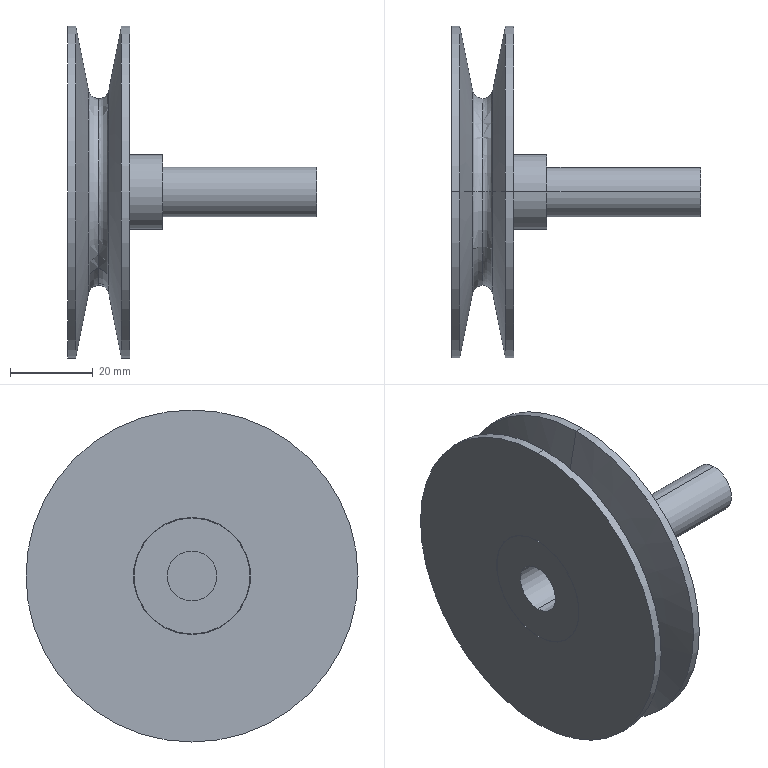Part | SolidWorks | features ICE 5, Revolution 1 | 1 solid | 35 faces | box 60 x 80 x 80 mm | volume 53043 mm3 | cylinder 18 | plane 9 | torus 4 | cone 4 | commonest cylinder face diameters 12 x4 28 x4 28.2 x4 80 x4 18 x2
STEP:
#1=CARTESIAN_POINT('',(5.047,0.,24.517));
#2=VERTEX_POINT('',#1);
#3=CARTESIAN_POINT('',(7.5,0.,22.5));
#4=VERTEX_POINT('',#3);
#5=CARTESIAN_POINT('',(7.5,0.,25.));
#6=DIRECTION('',(0.,-1.,0.));
#7=DIRECTION('',(0.,0.,-1.));
#8=AXIS2_PLACEMENT_3D('',#5,#6,#7);
#9=CIRCLE('',#8,2.5);
#10=EDGE_CURVE('',#2,#4,#9,.T.);
#11=ORIENTED_EDGE('',*,*,#10,.T.);
#12=CARTESIAN_POINT('',(7.5,0.,-22.5));
#13=VERTEX_POINT('',#12);
#14=CARTESIAN_POINT('',(7.5,0.,0.));
#15=DIRECTION('',(-1.,0.,0.));
#16=DIRECTION('',(0.,0.,1.));
#17=AXIS2_PLACEMENT_3D('',#14,#15,#16);
#18=CIRCLE('',#17,22.5);
#19=EDGE_CURVE('',#4,#13,#18,.T.);
#20=ORIENTED_EDGE('',*,*,#19,.T.);
#21=CARTESIAN_POINT('',(5.047,0.,-24.517));
#22=VERTEX_POINT('',#21);
#23=CARTESIAN_POINT('',(7.5,0.,-25.));
#24=DIRECTION('',(0.,1.,0.));
#25=DIRECTION('',(0.,0.,1.));
#26=AXIS2_PLACEMENT_3D('',#23,#24,#25);
#27=CIRCLE('',#26,2.5);
#28=EDGE_CURVE('',#22,#13,#27,.T.);
#29=ORIENTED_EDGE('',*,*,#28,.F.);
#30=CARTESIAN_POINT('',(5.047,0.,0.));
#31=DIRECTION('',(-1.,0.,0.));
#32=DIRECTION('',(0.,0.,1.));
#33=AXIS2_PLACEMENT_3D('',#30,#31,#32);
#34=CIRCLE('',#33,24.517);
#35=EDGE_CURVE('',#2,#22,#34,.T.);
#36=ORIENTED_EDGE('',*,*,#35,.F.);
#37=EDGE_LOOP('',(#11,#20,#29,#36));
#38=FACE_OUTER_BOUND('',#37,.T.);
#39=CARTESIAN_POINT('',(7.5,0.,0.));
#40=DIRECTION('',(-1.,0.,0.));
#41=DIRECTION('',(0.,0.,1.));
#42=AXIS2_PLACEMENT_3D('',#39,#40,#41);
#43=TOROIDAL_SURFACE('',#42,25.,2.5);
#44=ADVANCED_FACE('',(#38),#43,.F.);
#45=ORIENTED_EDGE('',*,*,#28,.T.);
#46=CARTESIAN_POINT('',(7.5,0.,0.));
#47=DIRECTION('',(-1.,0.,0.));
#48=DIRECTION('',(0.,0.,1.));
#49=AXIS2_PLACEMENT_3D('',#46,#47,#48);
#50=CIRCLE('',#49,22.5);
#51=EDGE_CURVE('',#13,#4,#50,.T.);
#52=ORIENTED_EDGE('',*,*,#51,.T.);
#53=ORIENTED_EDGE('',*,*,#10,.F.);
#54=CARTESIAN_POINT('',(5.047,0.,0.));
#55=DIRECTION('',(-1.,0.,0.));
#56=DIRECTION('',(0.,0.,1.));
#57=AXIS2_PLACEMENT_3D('',#54,#55,#56);
#58=CIRCLE('',#57,24.517);
#59=EDGE_CURVE('',#22,#2,#58,.T.);
#60=ORIENTED_EDGE('',*,*,#59,.F.);
#61=EDGE_LOOP('',(#45,#52,#53,#60));
#62=FACE_OUTER_BOUND('',#61,.T.);
#63=CARTESIAN_POINT('',(7.5,0.,0.));
#64=DIRECTION('',(-1.,0.,0.));
#65=DIRECTION('',(0.,0.,1.));
#66=AXIS2_PLACEMENT_3D('',#63,#64,#65);
#67=TOROIDAL_SURFACE('',#66,25.,2.5);
#68=ADVANCED_FACE('',(#62),#67,.F.);
#69=CARTESIAN_POINT('',(60.,0.,-6.));
#70=VERTEX_POINT('',#69);
#71=CARTESIAN_POINT('',(60.,0.,6.));
#72=VERTEX_POINT('',#71);
#73=CARTESIAN_POINT('',(60.,0.,0.));
#74=DIRECTION('',(1.,0.,0.));
#75=DIRECTION('',(0.,0.,-1.));
#76=AXIS2_PLACEMENT_3D('',#73,#74,#75);
#77=CIRCLE('',#76,6.);
#78=EDGE_CURVE('',#70,#72,#77,.T.);
#79=ORIENTED_EDGE('',*,*,#78,.F.);
#80=CARTESIAN_POINT('',(23.,0.,-6.));
#81=VERTEX_POINT('',#80);
#82=CARTESIAN_POINT('',(60.,0.,-6.));
#83=DIRECTION('',(-1.,0.,0.));
#84=VECTOR('',#83,1000.);
#85=LINE('',#82,#84);
#86=EDGE_CURVE('',#70,#81,#85,.T.);
#87=ORIENTED_EDGE('',*,*,#86,.T.);
#88=CARTESIAN_POINT('',(23.,0.,6.));
#89=VERTEX_POINT('',#88);
#90=CARTESIAN_POINT('',(23.,0.,0.));
#91=DIRECTION('',(-1.,0.,0.));
#92=DIRECTION('',(0.,0.,-1.));
#93=AXIS2_PLACEMENT_3D('',#90,#91,#92);
#94=CIRCLE('',#93,6.);
#95=EDGE_CURVE('',#89,#81,#94,.T.);
#96=ORIENTED_EDGE('',*,*,#95,.F.);
#97=CARTESIAN_POINT('',(60.,0.,6.));
#98=DIRECTION('',(-1.,0.,0.));
#99=VECTOR('',#98,1000.);
#100=LINE('',#97,#99);
#101=EDGE_CURVE('',#72,#89,#100,.T.);
#102=ORIENTED_EDGE('',*,*,#101,.F.);
#103=EDGE_LOOP('',(#79,#87,#96,#102));
#104=FACE_OUTER_BOUND('',#103,.T.);
#105=CARTESIAN_POINT('',(60.,0.,0.));
#106=DIRECTION('',(-1.,0.,0.));
#107=DIRECTION('',(0.,0.,1.));
#108=AXIS2_PLACEMENT_3D('',#105,#106,#107);
#109=CYLINDRICAL_SURFACE('',#108,6.);
#110=ADVANCED_FACE('',(#104),#109,.T.);
#111=CARTESIAN_POINT('',(23.,0.,-9.));
#112=VERTEX_POINT('',#111);
#113=CARTESIAN_POINT('',(23.,0.,9.));
#114=VERTEX_POINT('',#113);
#115=CARTESIAN_POINT('',(23.,0.,0.));
#116=DIRECTION('',(1.,0.,0.));
#117=DIRECTION('',(0.,0.,-1.));
#118=AXIS2_PLACEMENT_3D('',#115,#116,#117);
#119=CIRCLE('',#118,9.);
#120=EDGE_CURVE('',#112,#114,#119,.T.);
#121=ORIENTED_EDGE('',*,*,#120,.F.);
#122=CARTESIAN_POINT('',(15.,0.,-9.));
#123=VERTEX_POINT('',#122);
#124=CARTESIAN_POINT('',(23.,0.,-9.));
#125=DIRECTION('',(-1.,0.,0.));
#126=VECTOR('',#125,1000.);
#127=LINE('',#124,#126);
#128=EDGE_CURVE('',#112,#123,#127,.T.);
#129=ORIENTED_EDGE('',*,*,#128,.T.);
#130=CARTESIAN_POINT('',(15.,0.,9.));
#131=VERTEX_POINT('',#130);
#132=CARTESIAN_POINT('',(15.,0.,0.));
#133=DIRECTION('',(1.,0.,0.));
#134=DIRECTION('',(0.,0.,1.));
#135=AXIS2_PLACEMENT_3D('',#132,#133,#134);
#136=CIRCLE('',#135,9.);
#137=EDGE_CURVE('',#123,#131,#136,.T.);
#138=ORIENTED_EDGE('',*,*,#137,.T.);
#139=CARTESIAN_POINT('',(23.,0.,9.));
#140=DIRECTION('',(-1.,0.,0.));
#141=VECTOR('',#140,1000.);
#142=LINE('',#139,#141);
#143=EDGE_CURVE('',#114,#131,#142,.T.);
#144=ORIENTED_EDGE('',*,*,#143,.F.);
#145=EDGE_LOOP('',(#121,#129,#138,#144));
#146=FACE_OUTER_BOUND('',#145,.T.);
#147=CARTESIAN_POINT('',(23.,0.,0.));
#148=DIRECTION('',(-1.,0.,0.));
#149=DIRECTION('',(0.,0.,1.));
#150=AXIS2_PLACEMENT_3D('',#147,#148,#149);
#151=CYLINDRICAL_SURFACE('',#150,9.);
#152=ADVANCED_FACE('',(#146),#151,.T.);
#153=CARTESIAN_POINT('',(12.,0.,-14.));
#154=VERTEX_POINT('',#153);
#155=CARTESIAN_POINT('',(12.,0.,14.));
#156=VERTEX_POINT('',#155);
#157=CARTESIAN_POINT('',(12.,0.,0.));
#158=DIRECTION('',(1.,0.,0.));
#159=DIRECTION('',(0.,0.,-1.));
#160=AXIS2_PLACEMENT_3D('',#157,#158,#159);
#161=CIRCLE('',#160,14.);
#162=EDGE_CURVE('',#154,#156,#161,.T.);
#163=ORIENTED_EDGE('',*,*,#162,.T.);
#164=CARTESIAN_POINT('',(15.,0.,14.));
#165=VERTEX_POINT('',#164);
#166=CARTESIAN_POINT('',(12.,0.,14.));
#167=DIRECTION('',(1.,0.,0.));
#168=VECTOR('',#167,1000.);
#169=LINE('',#166,#168);
#170=EDGE_CURVE('',#156,#165,#169,.T.);
#171=ORIENTED_EDGE('',*,*,#170,.T.);
#172=CARTESIAN_POINT('',(15.,0.,-14.));
#173=VERTEX_POINT('',#172);
#174=CARTESIAN_POINT('',(15.,0.,0.));
#175=DIRECTION('',(1.,0.,0.));
#176=DIRECTION('',(0.,0.,-1.));
#177=AXIS2_PLACEMENT_3D('',#174,#175,#176);
#178=CIRCLE('',#177,14.);
#179=EDGE_CURVE('',#173,#165,#178,.T.);
#180=ORIENTED_EDGE('',*,*,#179,.F.);
#181=CARTESIAN_POINT('',(12.,0.,-14.));
#182=DIRECTION('',(1.,0.,0.));
#183=VECTOR('',#182,1000.);
#184=LINE('',#181,#183);
#185=EDGE_CURVE('',#154,#173,#184,.T.);
#186=ORIENTED_EDGE('',*,*,#185,.F.);
#187=EDGE_LOOP('',(#163,#171,#180,#186));
#188=FACE_OUTER_BOUND('',#187,.T.);
#189=CARTESIAN_POINT('',(12.,0.,0.));
#190=DIRECTION('',(1.,0.,0.));
#191=DIRECTION('',(0.,0.,-1.));
#192=AXIS2_PLACEMENT_3D('',#189,#190,#191);
#193=CYLINDRICAL_SURFACE('',#192,14.);
#194=ADVANCED_FACE('',(#188),#193,.T.);
#195=CARTESIAN_POINT('',(12.,0.,14.1));
#196=VERTEX_POINT('',#195);
#197=CARTESIAN_POINT('',(12.,0.,-14.1));
#198=VERTEX_POINT('',#197);
#199=CARTESIAN_POINT('',(12.,0.,0.));
#200=DIRECTION('',(1.,0.,0.));
#201=DIRECTION('',(0.,0.,-1.));
#202=AXIS2_PLACEMENT_3D('',#199,#200,#201);
#203=CIRCLE('',#202,14.1);
#204=EDGE_CURVE('',#196,#198,#203,.T.);
#205=ORIENTED_EDGE('',*,*,#204,.F.);
#206=CARTESIAN_POINT('',(15.,0.,14.1));
#207=VERTEX_POINT('',#206);
#208=CARTESIAN_POINT('',(12.,0.,14.1));
#209=DIRECTION('',(1.,0.,0.));
#210=VECTOR('',#209,1000.);
#211=LINE('',#208,#210);
#212=EDGE_CURVE('',#196,#207,#211,.T.);
#213=ORIENTED_EDGE('',*,*,#212,.T.);
#214=CARTESIAN_POINT('',(15.,0.,-14.1));
#215=VERTEX_POINT('',#214);
#216=CARTESIAN_POINT('',(15.,0.,0.));
#217=DIRECTION('',(1.,0.,0.));
#218=DIRECTION('',(0.,0.,-1.));
#219=AXIS2_PLACEMENT_3D('',#216,#217,#218);
#220=CIRCLE('',#219,14.1);
#221=EDGE_CURVE('',#207,#215,#220,.T.);
#222=ORIENTED_EDGE('',*,*,#221,.T.);
#223=CARTESIAN_POINT('',(12.,0.,-14.1));
#224=DIRECTION('',(1.,0.,0.));
#225=VECTOR('',#224,1000.);
#226=LINE('',#223,#225);
#227=EDGE_CURVE('',#198,#215,#226,.T.);
#228=ORIENTED_EDGE('',*,*,#227,.F.);
#229=EDGE_LOOP('',(#205,#213,#222,#228));
#230=FACE_OUTER_BOUND('',#229,.T.);
#231=CARTESIAN_POINT('',(12.,0.,0.));
#232=DIRECTION('',(1.,0.,0.));
#233=DIRECTION('',(0.,0.,-1.));
#234=AXIS2_PLACEMENT_3D('',#231,#232,#233);
#235=CYLINDRICAL_SURFACE('',#234,14.1);
#236=ADVANCED_FACE('',(#230),#235,.F.);
#237=CARTESIAN_POINT('',(3.,0.,14.));
#238=VERTEX_POINT('',#237);
#239=CARTESIAN_POINT('',(3.,0.,-14.));
#240=VERTEX_POINT('',#239);
#241=CARTESIAN_POINT('',(3.,0.,0.));
#242=DIRECTION('',(-1.,0.,0.));
#243=DIRECTION('',(0.,0.,1.));
#244=AXIS2_PLACEMENT_3D('',#241,#242,#243);
#245=CIRCLE('',#244,14.);
#246=EDGE_CURVE('',#238,#240,#245,.T.);
#247=ORIENTED_EDGE('',*,*,#246,.T.);
#248=CARTESIAN_POINT('',(0.,0.,-14.));
#249=VERTEX_POINT('',#248);
#250=CARTESIAN_POINT('',(3.,0.,-14.));
#251=DIRECTION('',(-1.,0.,0.));
#252=VECTOR('',#251,1000.);
#253=LINE('',#250,#252);
#254=EDGE_CURVE('',#240,#249,#253,.T.);
#255=ORIENTED_EDGE('',*,*,#254,.T.);
#256=CARTESIAN_POINT('',(0.,0.,14.));
#257=VERTEX_POINT('',#256);
#258=CARTESIAN_POINT('',(0.,0.,0.));
#259=DIRECTION('',(-1.,0.,0.));
#260=DIRECTION('',(0.,0.,1.));
#261=AXIS2_PLACEMENT_3D('',#258,#259,#260);
#262=CIRCLE('',#261,14.);
#263=EDGE_CURVE('',#257,#249,#262,.T.);
#264=ORIENTED_EDGE('',*,*,#263,.F.);
#265=CARTESIAN_POINT('',(3.,0.,14.));
#266=DIRECTION('',(-1.,0.,0.));
#267=VECTOR('',#266,1000.);
#268=LINE('',#265,#267);
#269=EDGE_CURVE('',#238,#257,#268,.T.);
#270=ORIENTED_EDGE('',*,*,#269,.F.);
#271=EDGE_LOOP('',(#247,#255,#264,#270));
#272=FACE_OUTER_BOUND('',#271,.T.);
#273=CARTESIAN_POINT('',(3.,0.,0.));
#274=DIRECTION('',(-1.,0.,0.));
#275=DIRECTION('',(0.,0.,1.));
#276=AXIS2_PLACEMENT_3D('',#273,#274,#275);
#277=CYLINDRICAL_SURFACE('',#276,14.);
#278=ADVANCED_FACE('',(#272),#277,.T.);
#279=CARTESIAN_POINT('',(3.,0.,-14.1));
#280=VERTEX_POINT('',#279);
#281=CARTESIAN_POINT('',(3.,0.,14.1));
#282=VERTEX_POINT('',#281);
#283=CARTESIAN_POINT('',(3.,0.,0.));
#284=DIRECTION('',(-1.,0.,0.));
#285=DIRECTION('',(0.,0.,1.));
#286=AXIS2_PLACEMENT_3D('',#283,#284,#285);
#287=CIRCLE('',#286,14.1);
#288=EDGE_CURVE('',#280,#282,#287,.T.);
#289=ORIENTED_EDGE('',*,*,#288,.F.);
#290=CARTESIAN_POINT('',(0.,0.,-14.1));
#291=VERTEX_POINT('',#290);
#292=CARTESIAN_POINT('',(3.,0.,-14.1));
#293=DIRECTION('',(-1.,0.,0.));
#294=VECTOR('',#293,1000.);
#295=LINE('',#292,#294);
#296=EDGE_CURVE('',#280,#291,#295,.T.);
#297=ORIENTED_EDGE('',*,*,#296,.T.);
#298=CARTESIAN_POINT('',(0.,0.,14.1));
#299=VERTEX_POINT('',#298);
#300=CARTESIAN_POINT('',(0.,0.,0.));
#301=DIRECTION('',(-1.,0.,0.));
#302=DIRECTION('',(0.,0.,1.));
#303=AXIS2_PLACEMENT_3D('',#300,#301,#302);
#304=CIRCLE('',#303,14.1);
#305=EDGE_CURVE('',#291,#299,#304,.T.);
#306=ORIENTED_EDGE('',*,*,#305,.T.);
#307=CARTESIAN_POINT('',(3.,0.,14.1));
#308=DIRECTION('',(-1.,0.,0.));
#309=VECTOR('',#308,1000.);
#310=LINE('',#307,#309);
#311=EDGE_CURVE('',#282,#299,#310,.T.);
#312=ORIENTED_EDGE('',*,*,#311,.F.);
#313=EDGE_LOOP('',(#289,#297,#306,#312));
#314=FACE_OUTER_BOUND('',#313,.T.);
#315=CARTESIAN_POINT('',(3.,0.,0.));
#316=DIRECTION('',(-1.,0.,0.));
#317=DIRECTION('',(0.,0.,1.));
#318=AXIS2_PLACEMENT_3D('',#315,#316,#317);
#319=CYLINDRICAL_SURFACE('',#318,14.1);
#320=ADVANCED_FACE('',(#314),#319,.F.);
#321=CARTESIAN_POINT('',(15.,0.,-6.));
#322=VERTEX_POINT('',#321);
#323=CARTESIAN_POINT('',(15.,0.,6.));
#324=VERTEX_POINT('',#323);
#325=CARTESIAN_POINT('',(15.,0.,0.));
#326=DIRECTION('',(-1.,0.,0.));
#327=DIRECTION('',(0.,0.,1.));
#328=AXIS2_PLACEMENT_3D('',#325,#326,#327);
#329=CIRCLE('',#328,6.);
#330=EDGE_CURVE('',#322,#324,#329,.T.);
#331=ORIENTED_EDGE('',*,*,#330,.F.);
#332=CARTESIAN_POINT('',(0.,0.,-6.));
#333=VERTEX_POINT('',#332);
#334=CARTESIAN_POINT('',(15.,0.,-6.));
#335=DIRECTION('',(-1.,0.,0.));
#336=VECTOR('',#335,1000.);
#337=LINE('',#334,#336);
#338=EDGE_CURVE('',#322,#333,#337,.T.);
#339=ORIENTED_EDGE('',*,*,#338,.T.);
#340=CARTESIAN_POINT('',(0.,0.,6.));
#341=VERTEX_POINT('',#340);
#342=CARTESIAN_POINT('',(0.,0.,0.));
#343=DIRECTION('',(-1.,0.,0.));
#344=DIRECTION('',(0.,0.,1.));
#345=AXIS2_PLACEMENT_3D('',#342,#343,#344);
#346=CIRCLE('',#345,6.);
#347=EDGE_CURVE('',#333,#341,#346,.T.);
#348=ORIENTED_EDGE('',*,*,#347,.T.);
#349=CARTESIAN_POINT('',(15.,0.,6.));
#350=DIRECTION('',(-1.,0.,0.));
#351=VECTOR('',#350,1000.);
#352=LINE('',#349,#351);
#353=EDGE_CURVE('',#324,#341,#352,.T.);
#354=ORIENTED_EDGE('',*,*,#353,.F.);
#355=EDGE_LOOP('',(#331,#339,#348,#354));
#356=FACE_OUTER_BOUND('',#355,.T.);
#357=CARTESIAN_POINT('',(15.,0.,0.));
#358=DIRECTION('',(-1.,0.,0.));
#359=DIRECTION('',(0.,0.,1.));
#360=AXIS2_PLACEMENT_3D('',#357,#358,#359);
#361=CYLINDRICAL_SURFACE('',#360,6.);
#362=ADVANCED_FACE('',(#356),#361,.F.);
#363=CARTESIAN_POINT('',(2.,0.,40.));
#364=VERTEX_POINT('',#363);
#365=CARTESIAN_POINT('',(2.,0.,-40.));
#366=VERTEX_POINT('',#365);
#367=CARTESIAN_POINT('',(2.,0.,0.));
#368=DIRECTION('',(-1.,0.,0.));
#369=DIRECTION('',(0.,0.,1.));
#370=AXIS2_PLACEMENT_3D('',#367,#368,#369);
#371=CIRCLE('',#370,40.);
#372=EDGE_CURVE('',#364,#366,#371,.T.);
#373=ORIENTED_EDGE('',*,*,#372,.T.);
#374=CARTESIAN_POINT('',(0.,0.,-40.));
#375=VERTEX_POINT('',#374);
#376=CARTESIAN_POINT('',(0.,0.,-40.));
#377=DIRECTION('',(-1.,0.,0.));
#378=VECTOR('',#377,1000.);
#379=LINE('',#376,#378);
#380=EDGE_CURVE('',#366,#375,#379,.T.);
#381=ORIENTED_EDGE('',*,*,#380,.T.);
#382=CARTESIAN_POINT('',(0.,0.,40.));
#383=VERTEX_POINT('',#382);
#384=CARTESIAN_POINT('',(0.,0.,0.));
#385=DIRECTION('',(-1.,0.,0.));
#386=DIRECTION('',(0.,0.,1.));
#387=AXIS2_PLACEMENT_3D('',#384,#385,#386);
#388=CIRCLE('',#387,40.);
#389=EDGE_CURVE('',#383,#375,#388,.T.);
#390=ORIENTED_EDGE('',*,*,#389,.F.);
#391=CARTESIAN_POINT('',(0.,0.,40.));
#392=DIRECTION('',(-1.,0.,0.));
#393=VECTOR('',#392,1000.);
#394=LINE('',#391,#393);
#395=EDGE_CURVE('',#364,#383,#394,.T.);
#396=ORIENTED_EDGE('',*,*,#395,.F.);
#397=EDGE_LOOP('',(#373,#381,#390,#396));
#398=FACE_OUTER_BOUND('',#397,.T.);
#399=CARTESIAN_POINT('',(0.,0.,0.));
#400=DIRECTION('',(-1.,0.,0.));
#401=DIRECTION('',(0.,0.,1.));
#402=AXIS2_PLACEMENT_3D('',#399,#400,#401);
#403=CYLINDRICAL_SURFACE('',#402,40.);
#404=ADVANCED_FACE('',(#398),#403,.T.);
#405=ORIENTED_EDGE('',*,*,#35,.T.);
#406=CARTESIAN_POINT('',(5.047,0.,-24.517));
#407=DIRECTION('',(-0.1931,0.,-0.9812));
#408=VECTOR('',#407,1000.);
#409=LINE('',#406,#408);
#410=EDGE_CURVE('',#22,#366,#409,.T.);
#411=ORIENTED_EDGE('',*,*,#410,.T.);
#412=ORIENTED_EDGE('',*,*,#372,.F.);
#413=CARTESIAN_POINT('',(5.047,0.,24.517));
#414=DIRECTION('',(-0.1931,0.,0.9812));
#415=VECTOR('',#414,1000.);
#416=LINE('',#413,#415);
#417=EDGE_CURVE('',#2,#364,#416,.T.);
#418=ORIENTED_EDGE('',*,*,#417,.F.);
#419=EDGE_LOOP('',(#405,#411,#412,#418));
#420=FACE_OUTER_BOUND('',#419,.T.);
#421=CARTESIAN_POINT('',(5.047,0.,0.));
#422=DIRECTION('',(-1.,0.,0.));
#423=DIRECTION('',(0.,0.,1.));
#424=AXIS2_PLACEMENT_3D('',#421,#422,#423);
#425=CONICAL_SURFACE('',#424,24.517,1.376);
#426=ADVANCED_FACE('',(#420),#425,.T.);
#427=ORIENTED_EDGE('',*,*,#51,.F.);
#428=CARTESIAN_POINT('',(9.953,0.,-24.517));
#429=VERTEX_POINT('',#428);
#430=CARTESIAN_POINT('',(7.5,0.,-25.));
#431=DIRECTION('',(0.,1.,0.));
#432=DIRECTION('',(0.,0.,1.));
#433=AXIS2_PLACEMENT_3D('',#430,#431,#432);
#434=CIRCLE('',#433,2.5);
#435=EDGE_CURVE('',#13,#429,#434,.T.);
#436=ORIENTED_EDGE('',*,*,#435,.T.);
#437=CARTESIAN_POINT('',(9.953,0.,24.517));
#438=VERTEX_POINT('',#437);
#439=CARTESIAN_POINT('',(9.953,0.,0.));
#440=DIRECTION('',(-1.,0.,0.));
#441=DIRECTION('',(0.,0.,1.));
#442=AXIS2_PLACEMENT_3D('',#439,#440,#441);
#443=CIRCLE('',#442,24.517);
#444=EDGE_CURVE('',#429,#438,#443,.T.);
#445=ORIENTED_EDGE('',*,*,#444,.T.);
#446=CARTESIAN_POINT('',(7.5,0.,25.));
#447=DIRECTION('',(0.,-1.,0.));
#448=DIRECTION('',(0.,0.,-1.));
#449=AXIS2_PLACEMENT_3D('',#446,#447,#448);
#450=CIRCLE('',#449,2.5);
#451=EDGE_CURVE('',#4,#438,#450,.T.);
#452=ORIENTED_EDGE('',*,*,#451,.F.);
#453=EDGE_LOOP('',(#427,#436,#445,#452));
#454=FACE_OUTER_BOUND('',#453,.T.);
#455=CARTESIAN_POINT('',(7.5,0.,0.));
#456=DIRECTION('',(-1.,0.,0.));
#457=DIRECTION('',(0.,0.,1.));
#458=AXIS2_PLACEMENT_3D('',#455,#456,#457);
#459=TOROIDAL_SURFACE('',#458,25.,2.5);
#460=ADVANCED_FACE('',(#454),#459,.F.);
#461=CARTESIAN_POINT('',(9.953,0.,0.));
#462=DIRECTION('',(-1.,0.,0.));
#463=DIRECTION('',(0.,0.,1.));
#464=AXIS2_PLACEMENT_3D('',#461,#462,#463);
#465=CIRCLE('',#464,24.517);
#466=EDGE_CURVE('',#438,#429,#465,.T.);
#467=ORIENTED_EDGE('',*,*,#466,.F.);
#468=CARTESIAN_POINT('',(13.,0.,40.));
#469=VERTEX_POINT('',#468);
#470=CARTESIAN_POINT('',(13.,0.,40.));
#471=DIRECTION('',(0.1931,0.,0.9812));
#472=VECTOR('',#471,1000.);
#473=LINE('',#470,#472);
#474=EDGE_CURVE('',#438,#469,#473,.T.);
#475=ORIENTED_EDGE('',*,*,#474,.T.);
#476=CARTESIAN_POINT('',(13.,0.,-40.));
#477=VERTEX_POINT('',#476);
#478=CARTESIAN_POINT('',(13.,0.,0.));
#479=DIRECTION('',(-1.,0.,0.));
#480=DIRECTION('',(0.,0.,1.));
#481=AXIS2_PLACEMENT_3D('',#478,#479,#480);
#482=CIRCLE('',#481,40.);
#483=EDGE_CURVE('',#469,#477,#482,.T.);
#484=ORIENTED_EDGE('',*,*,#483,.T.);
#485=CARTESIAN_POINT('',(13.,0.,-40.));
#486=DIRECTION('',(0.1931,0.,-0.9812));
#487=VECTOR('',#486,1000.);
#488=LINE('',#485,#487);
#489=EDGE_CURVE('',#429,#477,#488,.T.);
#490=ORIENTED_EDGE('',*,*,#489,.F.);
#491=EDGE_LOOP('',(#467,#475,#484,#490));
#492=FACE_OUTER_BOUND('',#491,.T.);
#493=CARTESIAN_POINT('',(13.,0.,0.));
#494=DIRECTION('',(1.,0.,0.));
#495=DIRECTION('',(0.,0.,-1.));
#496=AXIS2_PLACEMENT_3D('',#493,#494,#495);
#497=CONICAL_SURFACE('',#496,40.,1.376);
#498=ADVANCED_FACE('',(#492),#497,.T.);
#499=CARTESIAN_POINT('',(15.,0.,40.));
#500=VERTEX_POINT('',#499);
#501=CARTESIAN_POINT('',(15.,0.,-40.));
#502=VERTEX_POINT('',#501);
#503=CARTESIAN_POINT('',(15.,0.,0.));
#504=DIRECTION('',(-1.,0.,0.));
#505=DIRECTION('',(0.,0.,1.));
#506=AXIS2_PLACEMENT_3D('',#503,#504,#505);
#507=CIRCLE('',#506,40.);
#508=EDGE_CURVE('',#500,#502,#507,.T.);
#509=ORIENTED_EDGE('',*,*,#508,.T.);
#510=CARTESIAN_POINT('',(0.,0.,-40.));
#511=DIRECTION('',(-1.,0.,0.));
#512=VECTOR('',#511,1000.);
#513=LINE('',#510,#512);
#514=EDGE_CURVE('',#502,#477,#513,.T.);
#515=ORIENTED_EDGE('',*,*,#514,.T.);
#516=ORIENTED_EDGE('',*,*,#483,.F.);
#517=CARTESIAN_POINT('',(0.,0.,40.));
#518=DIRECTION('',(-1.,0.,0.));
#519=VECTOR('',#518,1000.);
#520=LINE('',#517,#519);
#521=EDGE_CURVE('',#500,#469,#520,.T.);
#522=ORIENTED_EDGE('',*,*,#521,.F.);
#523=EDGE_LOOP('',(#509,#515,#516,#522));
#524=FACE_OUTER_BOUND('',#523,.T.);
#525=CARTESIAN_POINT('',(0.,0.,0.));
#526=DIRECTION('',(-1.,0.,0.));
#527=DIRECTION('',(0.,0.,1.));
#528=AXIS2_PLACEMENT_3D('',#525,#526,#527);
#529=CYLINDRICAL_SURFACE('',#528,40.);
#530=ADVANCED_FACE('',(#524),#529,.T.);
#531=CARTESIAN_POINT('',(15.,0.,0.));
#532=DIRECTION('',(1.,0.,0.));
#533=DIRECTION('',(0.,0.,1.));
#534=AXIS2_PLACEMENT_3D('',#531,#532,#533);
#535=CIRCLE('',#534,9.);
#536=EDGE_CURVE('',#131,#123,#535,.T.);
#537=ORIENTED_EDGE('',*,*,#536,.F.);
#538=ORIENTED_EDGE('',*,*,#137,.F.);
#539=EDGE_LOOP('',(#537,#538));
#540=FACE_BOUND('',#539,.T.);
#541=ORIENTED_EDGE('',*,*,#179,.T.);
#542=CARTESIAN_POINT('',(15.,0.,0.));
#543=DIRECTION('',(1.,0.,0.));
#544=DIRECTION('',(0.,0.,-1.));
#545=AXIS2_PLACEMENT_3D('',#542,#543,#544);
#546=CIRCLE('',#545,14.);
#547=EDGE_CURVE('',#165,#173,#546,.T.);
#548=ORIENTED_EDGE('',*,*,#547,.T.);
#549=EDGE_LOOP('',(#541,#548));
#550=FACE_OUTER_BOUND('',#549,.T.);
#551=CARTESIAN_POINT('',(15.,40.,0.));
#552=DIRECTION('',(-1.,0.,0.));
#553=DIRECTION('',(0.,0.,1.));
#554=AXIS2_PLACEMENT_3D('',#551,#552,#553);
#555=PLANE('',#554);
#556=ADVANCED_FACE('',(#540,#550),#555,.F.);
#557=CARTESIAN_POINT('',(0.,0.,0.));
#558=DIRECTION('',(-1.,0.,0.));
#559=DIRECTION('',(0.,0.,1.));
#560=AXIS2_PLACEMENT_3D('',#557,#558,#559);
#561=CIRCLE('',#560,6.);
#562=EDGE_CURVE('',#341,#333,#561,.T.);
#563=ORIENTED_EDGE('',*,*,#562,.F.);
#564=ORIENTED_EDGE('',*,*,#347,.F.);
#565=EDGE_LOOP('',(#563,#564));
#566=FACE_BOUND('',#565,.T.);
#567=ORIENTED_EDGE('',*,*,#263,.T.);
#568=CARTESIAN_POINT('',(0.,0.,0.));
#569=DIRECTION('',(-1.,0.,0.));
#570=DIRECTION('',(0.,0.,1.));
#571=AXIS2_PLACEMENT_3D('',#568,#569,#570);
#572=CIRCLE('',#571,14.);
#573=EDGE_CURVE('',#249,#257,#572,.T.);
#574=ORIENTED_EDGE('',*,*,#573,.T.);
#575=EDGE_LOOP('',(#567,#574));
#576=FACE_OUTER_BOUND('',#575,.T.);
#577=CARTESIAN_POINT('',(0.,0.,0.));
#578=DIRECTION('',(1.,0.,0.));
#579=DIRECTION('',(0.,0.,-1.));
#580=AXIS2_PLACEMENT_3D('',#577,#578,#579);
#581=PLANE('',#580);
#582=ADVANCED_FACE('',(#566,#576),#581,.F.);
#583=CARTESIAN_POINT('',(15.,0.,0.));
#584=DIRECTION('',(1.,0.,0.));
#585=DIRECTION('',(0.,0.,-1.));
#586=AXIS2_PLACEMENT_3D('',#583,#584,#585);
#587=CIRCLE('',#586,14.1);
#588=EDGE_CURVE('',#215,#207,#587,.T.);
#589=ORIENTED_EDGE('',*,*,#588,.F.);
#590=ORIENTED_EDGE('',*,*,#221,.F.);
#591=EDGE_LOOP('',(#589,#590));
#592=FACE_BOUND('',#591,.T.);
#593=ORIENTED_EDGE('',*,*,#508,.F.);
#594=CARTESIAN_POINT('',(15.,0.,0.));
#595=DIRECTION('',(-1.,0.,0.));
#596=DIRECTION('',(0.,0.,1.));
#597=AXIS2_PLACEMENT_3D('',#594,#595,#596);
#598=CIRCLE('',#597,40.);
#599=EDGE_CURVE('',#502,#500,#598,.T.);
#600=ORIENTED_EDGE('',*,*,#599,.F.);
#601=EDGE_LOOP('',(#593,#600));
#602=FACE_OUTER_BOUND('',#601,.T.);
#603=CARTESIAN_POINT('',(15.,40.,0.));
#604=DIRECTION('',(-1.,0.,0.));
#605=DIRECTION('',(0.,0.,1.));
#606=AXIS2_PLACEMENT_3D('',#603,#604,#605);
#607=PLANE('',#606);
#608=ADVANCED_FACE('',(#592,#602),#607,.F.);
#609=ORIENTED_EDGE('',*,*,#514,.F.);
#610=ORIENTED_EDGE('',*,*,#599,.T.);
#611=ORIENTED_EDGE('',*,*,#521,.T.);
#612=CARTESIAN_POINT('',(13.,0.,0.));
#613=DIRECTION('',(-1.,0.,0.));
#614=DIRECTION('',(0.,0.,1.));
#615=AXIS2_PLACEMENT_3D('',#612,#613,#614);
#616=CIRCLE('',#615,40.);
#617=EDGE_CURVE('',#477,#469,#616,.T.);
#618=ORIENTED_EDGE('',*,*,#617,.F.);
#619=EDGE_LOOP('',(#609,#610,#611,#618));
#620=FACE_OUTER_BOUND('',#619,.T.);
#621=CARTESIAN_POINT('',(0.,0.,0.));
#622=DIRECTION('',(-1.,0.,0.));
#623=DIRECTION('',(0.,0.,1.));
#624=AXIS2_PLACEMENT_3D('',#621,#622,#623);
#625=CYLINDRICAL_SURFACE('',#624,40.);
#626=ADVANCED_FACE('',(#620),#625,.T.);
#627=ORIENTED_EDGE('',*,*,#474,.F.);
#628=ORIENTED_EDGE('',*,*,#444,.F.);
#629=ORIENTED_EDGE('',*,*,#489,.T.);
#630=ORIENTED_EDGE('',*,*,#617,.T.);
#631=EDGE_LOOP('',(#627,#628,#629,#630));
#632=FACE_OUTER_BOUND('',#631,.T.);
#633=CARTESIAN_POINT('',(13.,0.,0.));
#634=DIRECTION('',(1.,0.,0.));
#635=DIRECTION('',(0.,0.,-1.));
#636=AXIS2_PLACEMENT_3D('',#633,#634,#635);
#637=CONICAL_SURFACE('',#636,40.,1.376);
#638=ADVANCED_FACE('',(#632),#637,.T.);
#639=ORIENTED_EDGE('',*,*,#19,.F.);
#640=ORIENTED_EDGE('',*,*,#451,.T.);
#641=ORIENTED_EDGE('',*,*,#466,.T.);
#642=ORIENTED_EDGE('',*,*,#435,.F.);
#643=EDGE_LOOP('',(#639,#640,#641,#642));
#644=FACE_OUTER_BOUND('',#643,.T.);
#645=CARTESIAN_POINT('',(7.5,0.,0.));
#646=DIRECTION('',(-1.,0.,0.));
#647=DIRECTION('',(0.,0.,1.));
#648=AXIS2_PLACEMENT_3D('',#645,#646,#647);
#649=TOROIDAL_SURFACE('',#648,25.,2.5);
#650=ADVANCED_FACE('',(#644),#649,.F.);
#651=ORIENTED_EDGE('',*,*,#410,.F.);
#652=ORIENTED_EDGE('',*,*,#59,.T.);
#653=ORIENTED_EDGE('',*,*,#417,.T.);
#654=CARTESIAN_POINT('',(2.,0.,0.));
#655=DIRECTION('',(-1.,0.,0.));
#656=DIRECTION('',(0.,0.,1.));
#657=AXIS2_PLACEMENT_3D('',#654,#655,#656);
#658=CIRCLE('',#657,40.);
#659=EDGE_CURVE('',#366,#364,#658,.T.);
#660=ORIENTED_EDGE('',*,*,#659,.F.);
#661=EDGE_LOOP('',(#651,#652,#653,#660));
#662=FACE_OUTER_BOUND('',#661,.T.);
#663=CARTESIAN_POINT('',(5.047,0.,0.));
#664=DIRECTION('',(-1.,0.,0.));
#665=DIRECTION('',(0.,0.,1.));
#666=AXIS2_PLACEMENT_3D('',#663,#664,#665);
#667=CONICAL_SURFACE('',#666,24.517,1.376);
#668=ADVANCED_FACE('',(#662),#667,.T.);
#669=ORIENTED_EDGE('',*,*,#380,.F.);
#670=ORIENTED_EDGE('',*,*,#659,.T.);
#671=ORIENTED_EDGE('',*,*,#395,.T.);
#672=CARTESIAN_POINT('',(0.,0.,0.));
#673=DIRECTION('',(-1.,0.,0.));
#674=DIRECTION('',(0.,0.,1.));
#675=AXIS2_PLACEMENT_3D('',#672,#673,#674);
#676=CIRCLE('',#675,40.);
#677=EDGE_CURVE('',#375,#383,#676,.T.);
#678=ORIENTED_EDGE('',*,*,#677,.F.);
#679=EDGE_LOOP('',(#669,#670,#671,#678));
#680=FACE_OUTER_BOUND('',#679,.T.);
#681=CARTESIAN_POINT('',(0.,0.,0.));
#682=DIRECTION('',(-1.,0.,0.));
#683=DIRECTION('',(0.,0.,1.));
#684=AXIS2_PLACEMENT_3D('',#681,#682,#683);
#685=CYLINDRICAL_SURFACE('',#684,40.);
#686=ADVANCED_FACE('',(#680),#685,.T.);
#687=CARTESIAN_POINT('',(0.,0.,0.));
#688=DIRECTION('',(-1.,0.,0.));
#689=DIRECTION('',(0.,0.,1.));
#690=AXIS2_PLACEMENT_3D('',#687,#688,#689);
#691=CIRCLE('',#690,14.1);
#692=EDGE_CURVE('',#299,#291,#691,.T.);
#693=ORIENTED_EDGE('',*,*,#692,.F.);
#694=ORIENTED_EDGE('',*,*,#305,.F.);
#695=EDGE_LOOP('',(#693,#694));
#696=FACE_BOUND('',#695,.T.);
#697=ORIENTED_EDGE('',*,*,#389,.T.);
#698=ORIENTED_EDGE('',*,*,#677,.T.);
#699=EDGE_LOOP('',(#697,#698));
#700=FACE_OUTER_BOUND('',#699,.T.);
#701=CARTESIAN_POINT('',(0.,0.,0.));
#702=DIRECTION('',(1.,0.,0.));
#703=DIRECTION('',(0.,0.,-1.));
#704=AXIS2_PLACEMENT_3D('',#701,#702,#703);
#705=PLANE('',#704);
#706=ADVANCED_FACE('',(#696,#700),#705,.F.);
#707=ORIENTED_EDGE('',*,*,#338,.F.);
#708=CARTESIAN_POINT('',(15.,0.,0.));
#709=DIRECTION('',(-1.,0.,0.));
#710=DIRECTION('',(0.,0.,1.));
#711=AXIS2_PLACEMENT_3D('',#708,#709,#710);
#712=CIRCLE('',#711,6.);
#713=EDGE_CURVE('',#324,#322,#712,.T.);
#714=ORIENTED_EDGE('',*,*,#713,.F.);
#715=ORIENTED_EDGE('',*,*,#353,.T.);
#716=ORIENTED_EDGE('',*,*,#562,.T.);
#717=EDGE_LOOP('',(#707,#714,#715,#716));
#718=FACE_OUTER_BOUND('',#717,.T.);
#719=CARTESIAN_POINT('',(15.,0.,0.));
#720=DIRECTION('',(-1.,0.,0.));
#721=DIRECTION('',(0.,0.,1.));
#722=AXIS2_PLACEMENT_3D('',#719,#720,#721);
#723=CYLINDRICAL_SURFACE('',#722,6.);
#724=ADVANCED_FACE('',(#718),#723,.F.);
#725=ORIENTED_EDGE('',*,*,#296,.F.);
#726=CARTESIAN_POINT('',(3.,0.,0.));
#727=DIRECTION('',(-1.,0.,0.));
#728=DIRECTION('',(0.,0.,1.));
#729=AXIS2_PLACEMENT_3D('',#726,#727,#728);
#730=CIRCLE('',#729,14.1);
#731=EDGE_CURVE('',#282,#280,#730,.T.);
#732=ORIENTED_EDGE('',*,*,#731,.F.);
#733=ORIENTED_EDGE('',*,*,#311,.T.);
#734=ORIENTED_EDGE('',*,*,#692,.T.);
#735=EDGE_LOOP('',(#725,#732,#733,#734));
#736=FACE_OUTER_BOUND('',#735,.T.);
#737=CARTESIAN_POINT('',(3.,0.,0.));
#738=DIRECTION('',(-1.,0.,0.));
#739=DIRECTION('',(0.,0.,1.));
#740=AXIS2_PLACEMENT_3D('',#737,#738,#739);
#741=CYLINDRICAL_SURFACE('',#740,14.1);
#742=ADVANCED_FACE('',(#736),#741,.F.);
#743=ORIENTED_EDGE('',*,*,#246,.F.);
#744=CARTESIAN_POINT('',(3.,0.,0.));
#745=DIRECTION('',(-1.,0.,0.));
#746=DIRECTION('',(0.,0.,1.));
#747=AXIS2_PLACEMENT_3D('',#744,#745,#746);
#748=CIRCLE('',#747,14.);
#749=EDGE_CURVE('',#240,#238,#748,.T.);
#750=ORIENTED_EDGE('',*,*,#749,.F.);
#751=EDGE_LOOP('',(#743,#750));
#752=FACE_BOUND('',#751,.T.);
#753=ORIENTED_EDGE('',*,*,#731,.T.);
#754=ORIENTED_EDGE('',*,*,#288,.T.);
#755=EDGE_LOOP('',(#753,#754));
#756=FACE_OUTER_BOUND('',#755,.T.);
#757=CARTESIAN_POINT('',(3.,0.,0.));
#758=DIRECTION('',(-1.,0.,0.));
#759=DIRECTION('',(0.,0.,1.));
#760=AXIS2_PLACEMENT_3D('',#757,#758,#759);
#761=PLANE('',#760);
#762=ADVANCED_FACE('',(#752,#756),#761,.T.);
#763=ORIENTED_EDGE('',*,*,#254,.F.);
#764=ORIENTED_EDGE('',*,*,#749,.T.);
#765=ORIENTED_EDGE('',*,*,#269,.T.);
#766=ORIENTED_EDGE('',*,*,#573,.F.);
#767=EDGE_LOOP('',(#763,#764,#765,#766));
#768=FACE_OUTER_BOUND('',#767,.T.);
#769=CARTESIAN_POINT('',(3.,0.,0.));
#770=DIRECTION('',(-1.,0.,0.));
#771=DIRECTION('',(0.,0.,1.));
#772=AXIS2_PLACEMENT_3D('',#769,#770,#771);
#773=CYLINDRICAL_SURFACE('',#772,14.);
#774=ADVANCED_FACE('',(#768),#773,.T.);
#775=ORIENTED_EDGE('',*,*,#212,.F.);
#776=CARTESIAN_POINT('',(12.,0.,0.));
#777=DIRECTION('',(1.,0.,0.));
#778=DIRECTION('',(0.,0.,-1.));
#779=AXIS2_PLACEMENT_3D('',#776,#777,#778);
#780=CIRCLE('',#779,14.1);
#781=EDGE_CURVE('',#198,#196,#780,.T.);
#782=ORIENTED_EDGE('',*,*,#781,.F.);
#783=ORIENTED_EDGE('',*,*,#227,.T.);
#784=ORIENTED_EDGE('',*,*,#588,.T.);
#785=EDGE_LOOP('',(#775,#782,#783,#784));
#786=FACE_OUTER_BOUND('',#785,.T.);
#787=CARTESIAN_POINT('',(12.,0.,0.));
#788=DIRECTION('',(1.,0.,0.));
#789=DIRECTION('',(0.,0.,-1.));
#790=AXIS2_PLACEMENT_3D('',#787,#788,#789);
#791=CYLINDRICAL_SURFACE('',#790,14.1);
#792=ADVANCED_FACE('',(#786),#791,.F.);
#793=ORIENTED_EDGE('',*,*,#162,.F.);
#794=CARTESIAN_POINT('',(12.,0.,0.));
#795=DIRECTION('',(1.,0.,0.));
#796=DIRECTION('',(0.,0.,-1.));
#797=AXIS2_PLACEMENT_3D('',#794,#795,#796);
#798=CIRCLE('',#797,14.);
#799=EDGE_CURVE('',#156,#154,#798,.T.);
#800=ORIENTED_EDGE('',*,*,#799,.F.);
#801=EDGE_LOOP('',(#793,#800));
#802=FACE_BOUND('',#801,.T.);
#803=ORIENTED_EDGE('',*,*,#781,.T.);
#804=ORIENTED_EDGE('',*,*,#204,.T.);
#805=EDGE_LOOP('',(#803,#804));
#806=FACE_OUTER_BOUND('',#805,.T.);
#807=CARTESIAN_POINT('',(12.,0.,0.));
#808=DIRECTION('',(1.,0.,0.));
#809=DIRECTION('',(0.,0.,-1.));
#810=AXIS2_PLACEMENT_3D('',#807,#808,#809);
#811=PLANE('',#810);
#812=ADVANCED_FACE('',(#802,#806),#811,.T.);
#813=ORIENTED_EDGE('',*,*,#170,.F.);
#814=ORIENTED_EDGE('',*,*,#799,.T.);
#815=ORIENTED_EDGE('',*,*,#185,.T.);
#816=ORIENTED_EDGE('',*,*,#547,.F.);
#817=EDGE_LOOP('',(#813,#814,#815,#816));
#818=FACE_OUTER_BOUND('',#817,.T.);
#819=CARTESIAN_POINT('',(12.,0.,0.));
#820=DIRECTION('',(1.,0.,0.));
#821=DIRECTION('',(0.,0.,-1.));
#822=AXIS2_PLACEMENT_3D('',#819,#820,#821);
#823=CYLINDRICAL_SURFACE('',#822,14.);
#824=ADVANCED_FACE('',(#818),#823,.T.);
#825=ORIENTED_EDGE('',*,*,#713,.T.);
#826=ORIENTED_EDGE('',*,*,#330,.T.);
#827=EDGE_LOOP('',(#825,#826));
#828=FACE_OUTER_BOUND('',#827,.T.);
#829=CARTESIAN_POINT('',(15.,0.,0.));
#830=DIRECTION('',(1.,0.,0.));
#831=DIRECTION('',(0.,0.,-1.));
#832=AXIS2_PLACEMENT_3D('',#829,#830,#831);
#833=PLANE('',#832);
#834=ADVANCED_FACE('',(#828),#833,.F.);
#835=ORIENTED_EDGE('',*,*,#128,.F.);
#836=CARTESIAN_POINT('',(23.,0.,0.));
#837=DIRECTION('',(1.,0.,0.));
#838=DIRECTION('',(0.,0.,-1.));
#839=AXIS2_PLACEMENT_3D('',#836,#837,#838);
#840=CIRCLE('',#839,9.);
#841=EDGE_CURVE('',#114,#112,#840,.T.);
#842=ORIENTED_EDGE('',*,*,#841,.F.);
#843=ORIENTED_EDGE('',*,*,#143,.T.);
#844=ORIENTED_EDGE('',*,*,#536,.T.);
#845=EDGE_LOOP('',(#835,#842,#843,#844));
#846=FACE_OUTER_BOUND('',#845,.T.);
#847=CARTESIAN_POINT('',(23.,0.,0.));
#848=DIRECTION('',(-1.,0.,0.));
#849=DIRECTION('',(0.,0.,1.));
#850=AXIS2_PLACEMENT_3D('',#847,#848,#849);
#851=CYLINDRICAL_SURFACE('',#850,9.);
#852=ADVANCED_FACE('',(#846),#851,.T.);
#853=ORIENTED_EDGE('',*,*,#95,.T.);
#854=CARTESIAN_POINT('',(23.,0.,0.));
#855=DIRECTION('',(-1.,0.,0.));
#856=DIRECTION('',(0.,0.,-1.));
#857=AXIS2_PLACEMENT_3D('',#854,#855,#856);
#858=CIRCLE('',#857,6.);
#859=EDGE_CURVE('',#81,#89,#858,.T.);
#860=ORIENTED_EDGE('',*,*,#859,.T.);
#861=EDGE_LOOP('',(#853,#860));
#862=FACE_BOUND('',#861,.T.);
#863=ORIENTED_EDGE('',*,*,#841,.T.);
#864=ORIENTED_EDGE('',*,*,#120,.T.);
#865=EDGE_LOOP('',(#863,#864));
#866=FACE_OUTER_BOUND('',#865,.T.);
#867=CARTESIAN_POINT('',(23.,0.,0.));
#868=DIRECTION('',(1.,0.,0.));
#869=DIRECTION('',(0.,0.,-1.));
#870=AXIS2_PLACEMENT_3D('',#867,#868,#869);
#871=PLANE('',#870);
#872=ADVANCED_FACE('',(#862,#866),#871,.T.);
#873=ORIENTED_EDGE('',*,*,#86,.F.);
#874=CARTESIAN_POINT('',(60.,0.,0.));
#875=DIRECTION('',(1.,0.,0.));
#876=DIRECTION('',(0.,0.,-1.));
#877=AXIS2_PLACEMENT_3D('',#874,#875,#876);
#878=CIRCLE('',#877,6.);
#879=EDGE_CURVE('',#72,#70,#878,.T.);
#880=ORIENTED_EDGE('',*,*,#879,.F.);
#881=ORIENTED_EDGE('',*,*,#101,.T.);
#882=ORIENTED_EDGE('',*,*,#859,.F.);
#883=EDGE_LOOP('',(#873,#880,#881,#882));
#884=FACE_OUTER_BOUND('',#883,.T.);
#885=CARTESIAN_POINT('',(60.,0.,0.));
#886=DIRECTION('',(-1.,0.,0.));
#887=DIRECTION('',(0.,0.,1.));
#888=AXIS2_PLACEMENT_3D('',#885,#886,#887);
#889=CYLINDRICAL_SURFACE('',#888,6.);
#890=ADVANCED_FACE('',(#884),#889,.T.);
#891=ORIENTED_EDGE('',*,*,#879,.T.);
#892=ORIENTED_EDGE('',*,*,#78,.T.);
#893=EDGE_LOOP('',(#891,#892));
#894=FACE_OUTER_BOUND('',#893,.T.);
#895=CARTESIAN_POINT('',(60.,0.,0.));
#896=DIRECTION('',(1.,0.,0.));
#897=DIRECTION('',(0.,0.,-1.));
#898=AXIS2_PLACEMENT_3D('',#895,#896,#897);
#899=PLANE('',#898);
#900=ADVANCED_FACE('',(#894),#899,.T.);
#901=CLOSED_SHELL('',(#44,#68,#110,#152,#194,#236,#278,#320,#362,#404,#426,#460,#498,#530,#556,#582,#608,#626,#638,#650,#668,#686,#706,#724,#742,#762,#774,#792,#812,#824,#834,#852,#872,#890,#900));
#902=MANIFOLD_SOLID_BREP('',#901);
#903=CARTESIAN_POINT('',(0.,0.,0.));
#904=DIRECTION('',(0.,0.,1.));
#905=DIRECTION('',(1.,0.,0.));
#906=AXIS2_PLACEMENT_3D('',#903,#904,#905);
#907=(LENGTH_UNIT()NAMED_UNIT(*)SI_UNIT(.MILLI.,.METRE.));
#908=UNCERTAINTY_MEASURE_WITH_UNIT(LENGTH_MEASURE(0.00001),#907,'','');
#909=(NAMED_UNIT(*)PLANE_ANGLE_UNIT()SI_UNIT($,.RADIAN.));
#910=(NAMED_UNIT(*)SI_UNIT($,.STERADIAN.)SOLID_ANGLE_UNIT());
#911=(GEOMETRIC_REPRESENTATION_CONTEXT(3)GLOBAL_UNCERTAINTY_ASSIGNED_CONTEXT((#908))GLOBAL_UNIT_ASSIGNED_CONTEXT((#907,#909,#910))REPRESENTATION_CONTEXT('',''));
#912=ADVANCED_BREP_SHAPE_REPRESENTATION('',(#902,#906),#911);